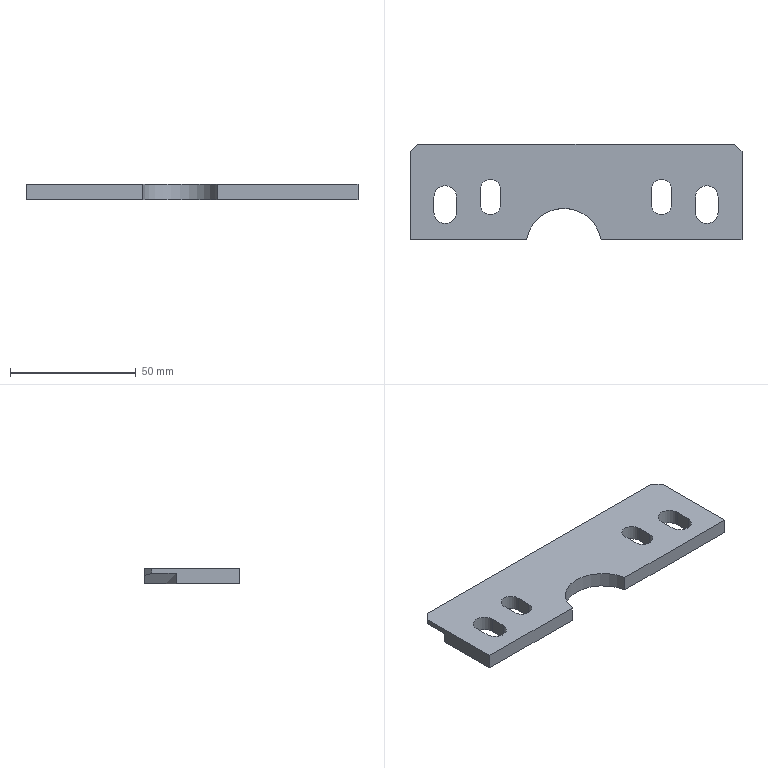Part | STEP file | gslz 2016.10.28-13_id726_x_t | 1 solid | 31 faces | box 132 x 38 x 6 mm | volume 25307 mm3 | plane 22 | cylinder 9 | commonest cylinder face diameters 8 x4 9 x4 30 x1